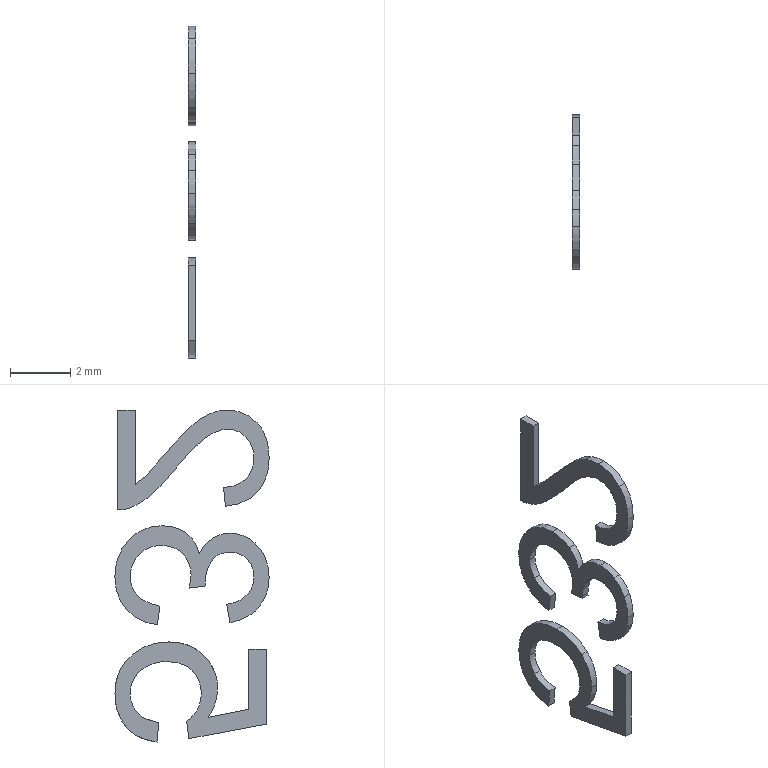Part | STEP file | BBS-JK-ZYBL-532-H5-1.stp.STEP | 3 solids | 80 faces | box 0.25 x 5.109 x 10.996 mm | volume 4.941 mm3 | spline 60 | plane 20